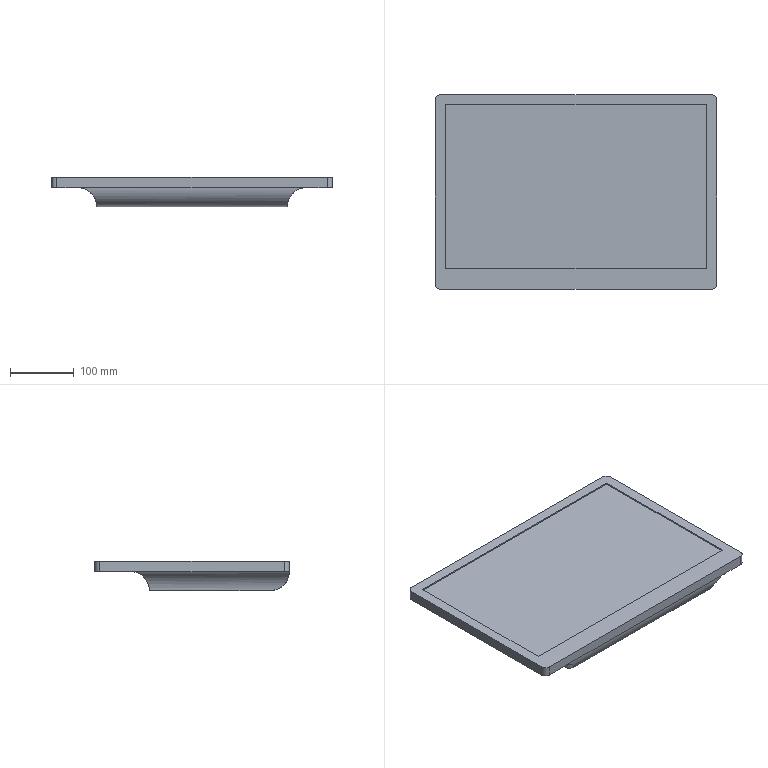Part | SolidWorks | features Fillet 3, ICE 2, Extrusion 1, HoleWzd 1 | 1 solid | 36 faces | box 442 x 306 x 46 mm | volume 4020857 mm3 | cylinder 16 | plane 12 | cone 8 | commonest cylinder face diameters 3.3 x8 16 x4 60 x4
STEP:
#1=CARTESIAN_POINT('',(51.65,41.,-19.9));
#2=VERTEX_POINT('',#1);
#3=CARTESIAN_POINT('',(48.35,41.,-19.9));
#4=VERTEX_POINT('',#3);
#5=CARTESIAN_POINT('',(50.,41.,-19.9));
#6=DIRECTION('',(0.,0.,-1.));
#7=DIRECTION('',(-1.,0.,0.));
#8=AXIS2_PLACEMENT_3D('',#5,#6,#7);
#9=CIRCLE('',#8,1.65);
#10=EDGE_CURVE('',#2,#4,#9,.T.);
#11=ORIENTED_EDGE('',*,*,#10,.F.);
#12=CARTESIAN_POINT('',(51.65,41.,-30.));
#13=VERTEX_POINT('',#12);
#14=CARTESIAN_POINT('',(51.65,41.,-30.));
#15=DIRECTION('',(0.,0.,-1.));
#16=VECTOR('',#15,1000.);
#17=LINE('',#14,#16);
#18=EDGE_CURVE('',#2,#13,#17,.T.);
#19=ORIENTED_EDGE('',*,*,#18,.T.);
#20=CARTESIAN_POINT('',(48.35,41.,-30.));
#21=VERTEX_POINT('',#20);
#22=CARTESIAN_POINT('',(50.,41.,-30.));
#23=DIRECTION('',(0.,0.,-1.));
#24=DIRECTION('',(-1.,0.,0.));
#25=AXIS2_PLACEMENT_3D('',#22,#23,#24);
#26=CIRCLE('',#25,1.65);
#27=EDGE_CURVE('',#13,#21,#26,.T.);
#28=ORIENTED_EDGE('',*,*,#27,.T.);
#29=CARTESIAN_POINT('',(48.35,41.,-30.));
#30=DIRECTION('',(0.,0.,-1.));
#31=VECTOR('',#30,1000.);
#32=LINE('',#29,#31);
#33=EDGE_CURVE('',#4,#21,#32,.T.);
#34=ORIENTED_EDGE('',*,*,#33,.F.);
#35=EDGE_LOOP('',(#11,#19,#28,#34));
#36=FACE_OUTER_BOUND('',#35,.T.);
#37=CARTESIAN_POINT('',(50.,41.,-30.));
#38=DIRECTION('',(0.,0.,-1.));
#39=DIRECTION('',(-1.,0.,0.));
#40=AXIS2_PLACEMENT_3D('',#37,#38,#39);
#41=CYLINDRICAL_SURFACE('',#40,1.65);
#42=ADVANCED_FACE('',(#36),#41,.F.);
#43=CARTESIAN_POINT('',(50.,41.,-18.909));
#44=VERTEX_POINT('',#43);
#45=CARTESIAN_POINT('',(48.35,41.,-19.9));
#46=DIRECTION('',(-0.8572,0.,-0.515));
#47=VECTOR('',#46,1000.);
#48=LINE('',#45,#47);
#49=EDGE_CURVE('',#44,#4,#48,.T.);
#50=ORIENTED_EDGE('',*,*,#49,.F.);
#51=CARTESIAN_POINT('',(51.65,41.,-19.9));
#52=DIRECTION('',(0.8572,0.,-0.515));
#53=VECTOR('',#52,1000.);
#54=LINE('',#51,#53);
#55=EDGE_CURVE('',#44,#2,#54,.T.);
#56=ORIENTED_EDGE('',*,*,#55,.T.);
#57=ORIENTED_EDGE('',*,*,#10,.T.);
#58=EDGE_LOOP('',(#50,#56,#57));
#59=FACE_OUTER_BOUND('',#58,.T.);
#60=CARTESIAN_POINT('',(50.,41.,-19.9));
#61=DIRECTION('',(0.,0.,-1.));
#62=DIRECTION('',(-1.,0.,0.));
#63=AXIS2_PLACEMENT_3D('',#60,#61,#62);
#64=CONICAL_SURFACE('',#63,1.65,1.03);
#65=ADVANCED_FACE('',(#59),#64,.F.);
#66=CARTESIAN_POINT('',(-48.35,41.,-19.9));
#67=VERTEX_POINT('',#66);
#68=CARTESIAN_POINT('',(-51.65,41.,-19.9));
#69=VERTEX_POINT('',#68);
#70=CARTESIAN_POINT('',(-50.,41.,-19.9));
#71=DIRECTION('',(0.,0.,-1.));
#72=DIRECTION('',(-1.,0.,0.));
#73=AXIS2_PLACEMENT_3D('',#70,#71,#72);
#74=CIRCLE('',#73,1.65);
#75=EDGE_CURVE('',#67,#69,#74,.T.);
#76=ORIENTED_EDGE('',*,*,#75,.F.);
#77=CARTESIAN_POINT('',(-48.35,41.,-30.));
#78=VERTEX_POINT('',#77);
#79=CARTESIAN_POINT('',(-48.35,41.,-30.));
#80=DIRECTION('',(0.,0.,-1.));
#81=VECTOR('',#80,1000.);
#82=LINE('',#79,#81);
#83=EDGE_CURVE('',#67,#78,#82,.T.);
#84=ORIENTED_EDGE('',*,*,#83,.T.);
#85=CARTESIAN_POINT('',(-51.65,41.,-30.));
#86=VERTEX_POINT('',#85);
#87=CARTESIAN_POINT('',(-50.,41.,-30.));
#88=DIRECTION('',(0.,0.,-1.));
#89=DIRECTION('',(-1.,0.,0.));
#90=AXIS2_PLACEMENT_3D('',#87,#88,#89);
#91=CIRCLE('',#90,1.65);
#92=EDGE_CURVE('',#78,#86,#91,.T.);
#93=ORIENTED_EDGE('',*,*,#92,.T.);
#94=CARTESIAN_POINT('',(-51.65,41.,-30.));
#95=DIRECTION('',(0.,0.,-1.));
#96=VECTOR('',#95,1000.);
#97=LINE('',#94,#96);
#98=EDGE_CURVE('',#69,#86,#97,.T.);
#99=ORIENTED_EDGE('',*,*,#98,.F.);
#100=EDGE_LOOP('',(#76,#84,#93,#99));
#101=FACE_OUTER_BOUND('',#100,.T.);
#102=CARTESIAN_POINT('',(-50.,41.,-30.));
#103=DIRECTION('',(0.,0.,-1.));
#104=DIRECTION('',(-1.,0.,0.));
#105=AXIS2_PLACEMENT_3D('',#102,#103,#104);
#106=CYLINDRICAL_SURFACE('',#105,1.65);
#107=ADVANCED_FACE('',(#101),#106,.F.);
#108=CARTESIAN_POINT('',(-50.,41.,-18.909));
#109=VERTEX_POINT('',#108);
#110=CARTESIAN_POINT('',(-51.65,41.,-19.9));
#111=DIRECTION('',(-0.8572,0.,-0.515));
#112=VECTOR('',#111,1000.);
#113=LINE('',#110,#112);
#114=EDGE_CURVE('',#109,#69,#113,.T.);
#115=ORIENTED_EDGE('',*,*,#114,.F.);
#116=CARTESIAN_POINT('',(-48.35,41.,-19.9));
#117=DIRECTION('',(0.8572,0.,-0.515));
#118=VECTOR('',#117,1000.);
#119=LINE('',#116,#118);
#120=EDGE_CURVE('',#109,#67,#119,.T.);
#121=ORIENTED_EDGE('',*,*,#120,.T.);
#122=ORIENTED_EDGE('',*,*,#75,.T.);
#123=EDGE_LOOP('',(#115,#121,#122));
#124=FACE_OUTER_BOUND('',#123,.T.);
#125=CARTESIAN_POINT('',(-50.,41.,-19.9));
#126=DIRECTION('',(0.,0.,-1.));
#127=DIRECTION('',(-1.,0.,0.));
#128=AXIS2_PLACEMENT_3D('',#125,#126,#127);
#129=CONICAL_SURFACE('',#128,1.65,1.03);
#130=ADVANCED_FACE('',(#124),#129,.F.);
#131=CARTESIAN_POINT('',(-48.35,-59.,-19.9));
#132=VERTEX_POINT('',#131);
#133=CARTESIAN_POINT('',(-51.65,-59.,-19.9));
#134=VERTEX_POINT('',#133);
#135=CARTESIAN_POINT('',(-50.,-59.,-19.9));
#136=DIRECTION('',(0.,0.,-1.));
#137=DIRECTION('',(-1.,0.,0.));
#138=AXIS2_PLACEMENT_3D('',#135,#136,#137);
#139=CIRCLE('',#138,1.65);
#140=EDGE_CURVE('',#132,#134,#139,.T.);
#141=ORIENTED_EDGE('',*,*,#140,.F.);
#142=CARTESIAN_POINT('',(-48.35,-59.,-30.));
#143=VERTEX_POINT('',#142);
#144=CARTESIAN_POINT('',(-48.35,-59.,-30.));
#145=DIRECTION('',(0.,0.,-1.));
#146=VECTOR('',#145,1000.);
#147=LINE('',#144,#146);
#148=EDGE_CURVE('',#132,#143,#147,.T.);
#149=ORIENTED_EDGE('',*,*,#148,.T.);
#150=CARTESIAN_POINT('',(-51.65,-59.,-30.));
#151=VERTEX_POINT('',#150);
#152=CARTESIAN_POINT('',(-50.,-59.,-30.));
#153=DIRECTION('',(0.,0.,-1.));
#154=DIRECTION('',(-1.,0.,0.));
#155=AXIS2_PLACEMENT_3D('',#152,#153,#154);
#156=CIRCLE('',#155,1.65);
#157=EDGE_CURVE('',#143,#151,#156,.T.);
#158=ORIENTED_EDGE('',*,*,#157,.T.);
#159=CARTESIAN_POINT('',(-51.65,-59.,-30.));
#160=DIRECTION('',(0.,0.,-1.));
#161=VECTOR('',#160,1000.);
#162=LINE('',#159,#161);
#163=EDGE_CURVE('',#134,#151,#162,.T.);
#164=ORIENTED_EDGE('',*,*,#163,.F.);
#165=EDGE_LOOP('',(#141,#149,#158,#164));
#166=FACE_OUTER_BOUND('',#165,.T.);
#167=CARTESIAN_POINT('',(-50.,-59.,-30.));
#168=DIRECTION('',(0.,0.,-1.));
#169=DIRECTION('',(-1.,0.,0.));
#170=AXIS2_PLACEMENT_3D('',#167,#168,#169);
#171=CYLINDRICAL_SURFACE('',#170,1.65);
#172=ADVANCED_FACE('',(#166),#171,.F.);
#173=CARTESIAN_POINT('',(-50.,-59.,-18.909));
#174=VERTEX_POINT('',#173);
#175=CARTESIAN_POINT('',(-51.65,-59.,-19.9));
#176=DIRECTION('',(-0.8572,0.,-0.515));
#177=VECTOR('',#176,1000.);
#178=LINE('',#175,#177);
#179=EDGE_CURVE('',#174,#134,#178,.T.);
#180=ORIENTED_EDGE('',*,*,#179,.F.);
#181=CARTESIAN_POINT('',(-48.35,-59.,-19.9));
#182=DIRECTION('',(0.8572,0.,-0.515));
#183=VECTOR('',#182,1000.);
#184=LINE('',#181,#183);
#185=EDGE_CURVE('',#174,#132,#184,.T.);
#186=ORIENTED_EDGE('',*,*,#185,.T.);
#187=ORIENTED_EDGE('',*,*,#140,.T.);
#188=EDGE_LOOP('',(#180,#186,#187));
#189=FACE_OUTER_BOUND('',#188,.T.);
#190=CARTESIAN_POINT('',(-50.,-59.,-19.9));
#191=DIRECTION('',(0.,0.,-1.));
#192=DIRECTION('',(-1.,0.,0.));
#193=AXIS2_PLACEMENT_3D('',#190,#191,#192);
#194=CONICAL_SURFACE('',#193,1.65,1.03);
#195=ADVANCED_FACE('',(#189),#194,.F.);
#196=CARTESIAN_POINT('',(51.65,-59.,-19.9));
#197=VERTEX_POINT('',#196);
#198=CARTESIAN_POINT('',(48.35,-59.,-19.9));
#199=VERTEX_POINT('',#198);
#200=CARTESIAN_POINT('',(50.,-59.,-19.9));
#201=DIRECTION('',(0.,0.,-1.));
#202=DIRECTION('',(-1.,0.,0.));
#203=AXIS2_PLACEMENT_3D('',#200,#201,#202);
#204=CIRCLE('',#203,1.65);
#205=EDGE_CURVE('',#197,#199,#204,.T.);
#206=ORIENTED_EDGE('',*,*,#205,.F.);
#207=CARTESIAN_POINT('',(51.65,-59.,-30.));
#208=VERTEX_POINT('',#207);
#209=CARTESIAN_POINT('',(51.65,-59.,-30.));
#210=DIRECTION('',(0.,0.,-1.));
#211=VECTOR('',#210,1000.);
#212=LINE('',#209,#211);
#213=EDGE_CURVE('',#197,#208,#212,.T.);
#214=ORIENTED_EDGE('',*,*,#213,.T.);
#215=CARTESIAN_POINT('',(48.35,-59.,-30.));
#216=VERTEX_POINT('',#215);
#217=CARTESIAN_POINT('',(50.,-59.,-30.));
#218=DIRECTION('',(0.,0.,-1.));
#219=DIRECTION('',(-1.,0.,0.));
#220=AXIS2_PLACEMENT_3D('',#217,#218,#219);
#221=CIRCLE('',#220,1.65);
#222=EDGE_CURVE('',#208,#216,#221,.T.);
#223=ORIENTED_EDGE('',*,*,#222,.T.);
#224=CARTESIAN_POINT('',(48.35,-59.,-30.));
#225=DIRECTION('',(0.,0.,-1.));
#226=VECTOR('',#225,1000.);
#227=LINE('',#224,#226);
#228=EDGE_CURVE('',#199,#216,#227,.T.);
#229=ORIENTED_EDGE('',*,*,#228,.F.);
#230=EDGE_LOOP('',(#206,#214,#223,#229));
#231=FACE_OUTER_BOUND('',#230,.T.);
#232=CARTESIAN_POINT('',(50.,-59.,-30.));
#233=DIRECTION('',(0.,0.,-1.));
#234=DIRECTION('',(-1.,0.,0.));
#235=AXIS2_PLACEMENT_3D('',#232,#233,#234);
#236=CYLINDRICAL_SURFACE('',#235,1.65);
#237=ADVANCED_FACE('',(#231),#236,.F.);
#238=CARTESIAN_POINT('',(50.,-59.,-18.909));
#239=VERTEX_POINT('',#238);
#240=CARTESIAN_POINT('',(48.35,-59.,-19.9));
#241=DIRECTION('',(-0.8572,0.,-0.515));
#242=VECTOR('',#241,1000.);
#243=LINE('',#240,#242);
#244=EDGE_CURVE('',#239,#199,#243,.T.);
#245=ORIENTED_EDGE('',*,*,#244,.F.);
#246=CARTESIAN_POINT('',(51.65,-59.,-19.9));
#247=DIRECTION('',(0.8572,0.,-0.515));
#248=VECTOR('',#247,1000.);
#249=LINE('',#246,#248);
#250=EDGE_CURVE('',#239,#197,#249,.T.);
#251=ORIENTED_EDGE('',*,*,#250,.T.);
#252=ORIENTED_EDGE('',*,*,#205,.T.);
#253=EDGE_LOOP('',(#245,#251,#252));
#254=FACE_OUTER_BOUND('',#253,.T.);
#255=CARTESIAN_POINT('',(50.,-59.,-19.9));
#256=DIRECTION('',(0.,0.,-1.));
#257=DIRECTION('',(-1.,0.,0.));
#258=AXIS2_PLACEMENT_3D('',#255,#256,#257);
#259=CONICAL_SURFACE('',#258,1.65,1.03);
#260=ADVANCED_FACE('',(#254),#259,.F.);
#261=CARTESIAN_POINT('',(-213.,-153.,0.));
#262=VERTEX_POINT('',#261);
#263=CARTESIAN_POINT('',(-180.,-153.,0.));
#264=VERTEX_POINT('',#263);
#265=CARTESIAN_POINT('',(-221.,-153.,0.));
#266=DIRECTION('',(1.,0.,0.));
#267=VECTOR('',#266,1000.);
#268=LINE('',#265,#267);
#269=EDGE_CURVE('',#262,#264,#268,.T.);
#270=ORIENTED_EDGE('',*,*,#269,.F.);
#271=CARTESIAN_POINT('',(-221.,-145.,0.));
#272=VERTEX_POINT('',#271);
#273=CARTESIAN_POINT('',(-213.,-145.,0.));
#274=DIRECTION('',(0.,0.,-1.));
#275=DIRECTION('',(1.,0.,0.));
#276=AXIS2_PLACEMENT_3D('',#273,#274,#275);
#277=CIRCLE('',#276,8.);
#278=EDGE_CURVE('',#262,#272,#277,.T.);
#279=ORIENTED_EDGE('',*,*,#278,.T.);
#280=CARTESIAN_POINT('',(-221.,145.,0.));
#281=VERTEX_POINT('',#280);
#282=CARTESIAN_POINT('',(-221.,153.,0.));
#283=DIRECTION('',(0.,-1.,0.));
#284=VECTOR('',#283,1000.);
#285=LINE('',#282,#284);
#286=EDGE_CURVE('',#281,#272,#285,.T.);
#287=ORIENTED_EDGE('',*,*,#286,.F.);
#288=CARTESIAN_POINT('',(-213.,153.,0.));
#289=VERTEX_POINT('',#288);
#290=CARTESIAN_POINT('',(-213.,145.,0.));
#291=DIRECTION('',(0.,0.,-1.));
#292=DIRECTION('',(1.,0.,0.));
#293=AXIS2_PLACEMENT_3D('',#290,#291,#292);
#294=CIRCLE('',#293,8.);
#295=EDGE_CURVE('',#281,#289,#294,.T.);
#296=ORIENTED_EDGE('',*,*,#295,.T.);
#297=CARTESIAN_POINT('',(213.,153.,0.));
#298=VERTEX_POINT('',#297);
#299=CARTESIAN_POINT('',(-221.,153.,0.));
#300=DIRECTION('',(-1.,0.,0.));
#301=VECTOR('',#300,1000.);
#302=LINE('',#299,#301);
#303=EDGE_CURVE('',#298,#289,#302,.T.);
#304=ORIENTED_EDGE('',*,*,#303,.F.);
#305=CARTESIAN_POINT('',(221.,145.,0.));
#306=VERTEX_POINT('',#305);
#307=CARTESIAN_POINT('',(213.,145.,0.));
#308=DIRECTION('',(0.,0.,-1.));
#309=DIRECTION('',(1.,0.,0.));
#310=AXIS2_PLACEMENT_3D('',#307,#308,#309);
#311=CIRCLE('',#310,8.);
#312=EDGE_CURVE('',#298,#306,#311,.T.);
#313=ORIENTED_EDGE('',*,*,#312,.T.);
#314=CARTESIAN_POINT('',(221.,-145.,0.));
#315=VERTEX_POINT('',#314);
#316=CARTESIAN_POINT('',(221.,153.,0.));
#317=DIRECTION('',(0.,1.,0.));
#318=VECTOR('',#317,1000.);
#319=LINE('',#316,#318);
#320=EDGE_CURVE('',#315,#306,#319,.T.);
#321=ORIENTED_EDGE('',*,*,#320,.F.);
#322=CARTESIAN_POINT('',(213.,-153.,0.));
#323=VERTEX_POINT('',#322);
#324=CARTESIAN_POINT('',(213.,-145.,0.));
#325=DIRECTION('',(0.,0.,-1.));
#326=DIRECTION('',(1.,0.,0.));
#327=AXIS2_PLACEMENT_3D('',#324,#325,#326);
#328=CIRCLE('',#327,8.);
#329=EDGE_CURVE('',#315,#323,#328,.T.);
#330=ORIENTED_EDGE('',*,*,#329,.T.);
#331=CARTESIAN_POINT('',(180.,-153.,0.));
#332=VERTEX_POINT('',#331);
#333=CARTESIAN_POINT('',(-221.,-153.,0.));
#334=DIRECTION('',(1.,0.,0.));
#335=VECTOR('',#334,1000.);
#336=LINE('',#333,#335);
#337=EDGE_CURVE('',#332,#323,#336,.T.);
#338=ORIENTED_EDGE('',*,*,#337,.F.);
#339=CARTESIAN_POINT('',(180.,97.,0.));
#340=VERTEX_POINT('',#339);
#341=CARTESIAN_POINT('',(180.,67.,0.));
#342=DIRECTION('',(0.,1.,0.));
#343=VECTOR('',#342,1000.);
#344=LINE('',#341,#343);
#345=EDGE_CURVE('',#332,#340,#344,.T.);
#346=ORIENTED_EDGE('',*,*,#345,.T.);
#347=CARTESIAN_POINT('',(-180.,97.,0.));
#348=VERTEX_POINT('',#347);
#349=CARTESIAN_POINT('',(-150.,97.,0.));
#350=DIRECTION('',(-1.,0.,0.));
#351=VECTOR('',#350,1000.);
#352=LINE('',#349,#351);
#353=EDGE_CURVE('',#340,#348,#352,.T.);
#354=ORIENTED_EDGE('',*,*,#353,.T.);
#355=CARTESIAN_POINT('',(-180.,-153.,0.));
#356=DIRECTION('',(0.,-1.,0.));
#357=VECTOR('',#356,1000.);
#358=LINE('',#355,#357);
#359=EDGE_CURVE('',#348,#264,#358,.T.);
#360=ORIENTED_EDGE('',*,*,#359,.T.);
#361=EDGE_LOOP('',(#270,#279,#287,#296,#304,#313,#321,#330,#338,#346,#354,#360));
#362=FACE_OUTER_BOUND('',#361,.T.);
#363=CARTESIAN_POINT('',(0.,0.,0.));
#364=DIRECTION('',(0.,0.,1.));
#365=DIRECTION('',(1.,0.,0.));
#366=AXIS2_PLACEMENT_3D('',#363,#364,#365);
#367=PLANE('',#366);
#368=ADVANCED_FACE('',(#362),#367,.F.);
#369=CARTESIAN_POINT('',(221.,-145.,16.));
#370=VERTEX_POINT('',#369);
#371=CARTESIAN_POINT('',(221.,145.,16.));
#372=VERTEX_POINT('',#371);
#373=CARTESIAN_POINT('',(221.,153.,16.));
#374=DIRECTION('',(0.,1.,0.));
#375=VECTOR('',#374,1000.);
#376=LINE('',#373,#375);
#377=EDGE_CURVE('',#370,#372,#376,.T.);
#378=ORIENTED_EDGE('',*,*,#377,.F.);
#379=CARTESIAN_POINT('',(221.,-145.,16.));
#380=DIRECTION('',(0.,0.,-1.));
#381=VECTOR('',#380,1000.);
#382=LINE('',#379,#381);
#383=EDGE_CURVE('',#370,#315,#382,.T.);
#384=ORIENTED_EDGE('',*,*,#383,.T.);
#385=ORIENTED_EDGE('',*,*,#320,.T.);
#386=CARTESIAN_POINT('',(221.,145.,16.));
#387=DIRECTION('',(0.,0.,1.));
#388=VECTOR('',#387,1000.);
#389=LINE('',#386,#388);
#390=EDGE_CURVE('',#306,#372,#389,.T.);
#391=ORIENTED_EDGE('',*,*,#390,.T.);
#392=EDGE_LOOP('',(#378,#384,#385,#391));
#393=FACE_OUTER_BOUND('',#392,.T.);
#394=CARTESIAN_POINT('',(221.,153.,16.));
#395=DIRECTION('',(-1.,0.,0.));
#396=DIRECTION('',(0.,-1.,0.));
#397=AXIS2_PLACEMENT_3D('',#394,#395,#396);
#398=PLANE('',#397);
#399=ADVANCED_FACE('',(#393),#398,.F.);
#400=CARTESIAN_POINT('',(213.,153.,16.));
#401=VERTEX_POINT('',#400);
#402=CARTESIAN_POINT('',(-213.,153.,16.));
#403=VERTEX_POINT('',#402);
#404=CARTESIAN_POINT('',(-221.,153.,16.));
#405=DIRECTION('',(-1.,0.,0.));
#406=VECTOR('',#405,1000.);
#407=LINE('',#404,#406);
#408=EDGE_CURVE('',#401,#403,#407,.T.);
#409=ORIENTED_EDGE('',*,*,#408,.F.);
#410=CARTESIAN_POINT('',(213.,153.,16.));
#411=DIRECTION('',(0.,0.,-1.));
#412=VECTOR('',#411,1000.);
#413=LINE('',#410,#412);
#414=EDGE_CURVE('',#401,#298,#413,.T.);
#415=ORIENTED_EDGE('',*,*,#414,.T.);
#416=ORIENTED_EDGE('',*,*,#303,.T.);
#417=CARTESIAN_POINT('',(-213.,153.,16.));
#418=DIRECTION('',(0.,0.,1.));
#419=VECTOR('',#418,1000.);
#420=LINE('',#417,#419);
#421=EDGE_CURVE('',#289,#403,#420,.T.);
#422=ORIENTED_EDGE('',*,*,#421,.T.);
#423=EDGE_LOOP('',(#409,#415,#416,#422));
#424=FACE_OUTER_BOUND('',#423,.T.);
#425=CARTESIAN_POINT('',(-221.,153.,16.));
#426=DIRECTION('',(0.,-1.,0.));
#427=DIRECTION('',(0.,0.,-1.));
#428=AXIS2_PLACEMENT_3D('',#425,#426,#427);
#429=PLANE('',#428);
#430=ADVANCED_FACE('',(#424),#429,.F.);
#431=ORIENTED_EDGE('',*,*,#286,.T.);
#432=CARTESIAN_POINT('',(-221.,-145.,16.));
#433=VERTEX_POINT('',#432);
#434=CARTESIAN_POINT('',(-221.,-145.,16.));
#435=DIRECTION('',(0.,0.,1.));
#436=VECTOR('',#435,1000.);
#437=LINE('',#434,#436);
#438=EDGE_CURVE('',#272,#433,#437,.T.);
#439=ORIENTED_EDGE('',*,*,#438,.T.);
#440=CARTESIAN_POINT('',(-221.,145.,16.));
#441=VERTEX_POINT('',#440);
#442=CARTESIAN_POINT('',(-221.,153.,16.));
#443=DIRECTION('',(0.,-1.,0.));
#444=VECTOR('',#443,1000.);
#445=LINE('',#442,#444);
#446=EDGE_CURVE('',#441,#433,#445,.T.);
#447=ORIENTED_EDGE('',*,*,#446,.F.);
#448=CARTESIAN_POINT('',(-221.,145.,16.));
#449=DIRECTION('',(0.,0.,-1.));
#450=VECTOR('',#449,1000.);
#451=LINE('',#448,#450);
#452=EDGE_CURVE('',#441,#281,#451,.T.);
#453=ORIENTED_EDGE('',*,*,#452,.T.);
#454=EDGE_LOOP('',(#431,#439,#447,#453));
#455=FACE_OUTER_BOUND('',#454,.T.);
#456=CARTESIAN_POINT('',(-221.,153.,16.));
#457=DIRECTION('',(1.,0.,0.));
#458=DIRECTION('',(0.,1.,0.));
#459=AXIS2_PLACEMENT_3D('',#456,#457,#458);
#460=PLANE('',#459);
#461=ADVANCED_FACE('',(#455),#460,.F.);
#462=CARTESIAN_POINT('',(-213.,-153.,16.));
#463=VERTEX_POINT('',#462);
#464=CARTESIAN_POINT('',(213.,-153.,16.));
#465=VERTEX_POINT('',#464);
#466=CARTESIAN_POINT('',(-221.,-153.,16.));
#467=DIRECTION('',(1.,0.,0.));
#468=VECTOR('',#467,1000.);
#469=LINE('',#466,#468);
#470=EDGE_CURVE('',#463,#465,#469,.T.);
#471=ORIENTED_EDGE('',*,*,#470,.F.);
#472=CARTESIAN_POINT('',(-213.,-153.,16.));
#473=DIRECTION('',(0.,0.,-1.));
#474=VECTOR('',#473,1000.);
#475=LINE('',#472,#474);
#476=EDGE_CURVE('',#463,#262,#475,.T.);
#477=ORIENTED_EDGE('',*,*,#476,.T.);
#478=ORIENTED_EDGE('',*,*,#269,.T.);
#479=CARTESIAN_POINT('',(-221.,-153.,0.));
#480=DIRECTION('',(1.,0.,0.));
#481=VECTOR('',#480,1000.);
#482=LINE('',#479,#481);
#483=EDGE_CURVE('',#264,#332,#482,.T.);
#484=ORIENTED_EDGE('',*,*,#483,.T.);
#485=ORIENTED_EDGE('',*,*,#337,.T.);
#486=CARTESIAN_POINT('',(213.,-153.,16.));
#487=DIRECTION('',(0.,0.,1.));
#488=VECTOR('',#487,1000.);
#489=LINE('',#486,#488);
#490=EDGE_CURVE('',#323,#465,#489,.T.);
#491=ORIENTED_EDGE('',*,*,#490,.T.);
#492=EDGE_LOOP('',(#471,#477,#478,#484,#485,#491));
#493=FACE_OUTER_BOUND('',#492,.T.);
#494=CARTESIAN_POINT('',(-221.,-153.,16.));
#495=DIRECTION('',(0.,1.,0.));
#496=DIRECTION('',(0.,0.,1.));
#497=AXIS2_PLACEMENT_3D('',#494,#495,#496);
#498=PLANE('',#497);
#499=ADVANCED_FACE('',(#493),#498,.F.);
#500=CARTESIAN_POINT('',(205.,-121.,16.));
#501=VERTEX_POINT('',#500);
#502=CARTESIAN_POINT('',(205.,137.,16.));
#503=VERTEX_POINT('',#502);
#504=CARTESIAN_POINT('',(205.,137.,16.));
#505=DIRECTION('',(0.,1.,0.));
#506=VECTOR('',#505,1000.);
#507=LINE('',#504,#506);
#508=EDGE_CURVE('',#501,#503,#507,.T.);
#509=ORIENTED_EDGE('',*,*,#508,.F.);
#510=CARTESIAN_POINT('',(-205.,-121.,16.));
#511=VERTEX_POINT('',#510);
#512=CARTESIAN_POINT('',(-205.,-121.,16.));
#513=DIRECTION('',(1.,0.,0.));
#514=VECTOR('',#513,1000.);
#515=LINE('',#512,#514);
#516=EDGE_CURVE('',#511,#501,#515,.T.);
#517=ORIENTED_EDGE('',*,*,#516,.F.);
#518=CARTESIAN_POINT('',(-205.,137.,16.));
#519=VERTEX_POINT('',#518);
#520=CARTESIAN_POINT('',(-205.,137.,16.));
#521=DIRECTION('',(0.,-1.,0.));
#522=VECTOR('',#521,1000.);
#523=LINE('',#520,#522);
#524=EDGE_CURVE('',#519,#511,#523,.T.);
#525=ORIENTED_EDGE('',*,*,#524,.F.);
#526=CARTESIAN_POINT('',(-205.,137.,16.));
#527=DIRECTION('',(-1.,0.,0.));
#528=VECTOR('',#527,1000.);
#529=LINE('',#526,#528);
#530=EDGE_CURVE('',#503,#519,#529,.T.);
#531=ORIENTED_EDGE('',*,*,#530,.F.);
#532=EDGE_LOOP('',(#509,#517,#525,#531));
#533=FACE_BOUND('',#532,.T.);
#534=ORIENTED_EDGE('',*,*,#446,.T.);
#535=CARTESIAN_POINT('',(-213.,-145.,16.));
#536=DIRECTION('',(0.,0.,1.));
#537=DIRECTION('',(1.,0.,0.));
#538=AXIS2_PLACEMENT_3D('',#535,#536,#537);
#539=CIRCLE('',#538,8.);
#540=EDGE_CURVE('',#433,#463,#539,.T.);
#541=ORIENTED_EDGE('',*,*,#540,.T.);
#542=ORIENTED_EDGE('',*,*,#470,.T.);
#543=CARTESIAN_POINT('',(213.,-145.,16.));
#544=DIRECTION('',(0.,0.,1.));
#545=DIRECTION('',(1.,0.,0.));
#546=AXIS2_PLACEMENT_3D('',#543,#544,#545);
#547=CIRCLE('',#546,8.);
#548=EDGE_CURVE('',#465,#370,#547,.T.);
#549=ORIENTED_EDGE('',*,*,#548,.T.);
#550=ORIENTED_EDGE('',*,*,#377,.T.);
#551=CARTESIAN_POINT('',(213.,145.,16.));
#552=DIRECTION('',(0.,0.,1.));
#553=DIRECTION('',(1.,0.,0.));
#554=AXIS2_PLACEMENT_3D('',#551,#552,#553);
#555=CIRCLE('',#554,8.);
#556=EDGE_CURVE('',#372,#401,#555,.T.);
#557=ORIENTED_EDGE('',*,*,#556,.T.);
#558=ORIENTED_EDGE('',*,*,#408,.T.);
#559=CARTESIAN_POINT('',(-213.,145.,16.));
#560=DIRECTION('',(0.,0.,1.));
#561=DIRECTION('',(1.,0.,0.));
#562=AXIS2_PLACEMENT_3D('',#559,#560,#561);
#563=CIRCLE('',#562,8.);
#564=EDGE_CURVE('',#403,#441,#563,.T.);
#565=ORIENTED_EDGE('',*,*,#564,.T.);
#566=EDGE_LOOP('',(#534,#541,#542,#549,#550,#557,#558,#565));
#567=FACE_OUTER_BOUND('',#566,.T.);
#568=CARTESIAN_POINT('',(0.,0.,16.));
#569=DIRECTION('',(0.,0.,1.));
#570=DIRECTION('',(1.,0.,0.));
#571=AXIS2_PLACEMENT_3D('',#568,#569,#570);
#572=PLANE('',#571);
#573=ADVANCED_FACE('',(#533,#567),#572,.T.);
#574=CARTESIAN_POINT('',(50.,41.,-30.));
#575=DIRECTION('',(0.,0.,-1.));
#576=DIRECTION('',(-1.,0.,0.));
#577=AXIS2_PLACEMENT_3D('',#574,#575,#576);
#578=CIRCLE('',#577,1.65);
#579=EDGE_CURVE('',#21,#13,#578,.T.);
#580=ORIENTED_EDGE('',*,*,#579,.F.);
#581=ORIENTED_EDGE('',*,*,#27,.F.);
#582=EDGE_LOOP('',(#580,#581));
#583=FACE_BOUND('',#582,.T.);
#584=CARTESIAN_POINT('',(-50.,41.,-30.));
#585=DIRECTION('',(0.,0.,-1.));
#586=DIRECTION('',(-1.,0.,0.));
#587=AXIS2_PLACEMENT_3D('',#584,#585,#586);
#588=CIRCLE('',#587,1.65);
#589=EDGE_CURVE('',#86,#78,#588,.T.);
#590=ORIENTED_EDGE('',*,*,#589,.F.);
#591=ORIENTED_EDGE('',*,*,#92,.F.);
#592=EDGE_LOOP('',(#590,#591));
#593=FACE_BOUND('',#592,.T.);
#594=CARTESIAN_POINT('',(-50.,-59.,-30.));
#595=DIRECTION('',(0.,0.,-1.));
#596=DIRECTION('',(-1.,0.,0.));
#597=AXIS2_PLACEMENT_3D('',#594,#595,#596);
#598=CIRCLE('',#597,1.65);
#599=EDGE_CURVE('',#151,#143,#598,.T.);
#600=ORIENTED_EDGE('',*,*,#599,.F.);
#601=ORIENTED_EDGE('',*,*,#157,.F.);
#602=EDGE_LOOP('',(#600,#601));
#603=FACE_BOUND('',#602,.T.);
#604=CARTESIAN_POINT('',(50.,-59.,-30.));
#605=DIRECTION('',(0.,0.,-1.));
#606=DIRECTION('',(-1.,0.,0.));
#607=AXIS2_PLACEMENT_3D('',#604,#605,#606);
#608=CIRCLE('',#607,1.65);
#609=EDGE_CURVE('',#216,#208,#608,.T.);
#610=ORIENTED_EDGE('',*,*,#609,.F.);
#611=ORIENTED_EDGE('',*,*,#222,.F.);
#612=EDGE_LOOP('',(#610,#611));
#613=FACE_BOUND('',#612,.T.);
#614=CARTESIAN_POINT('',(150.,67.,-30.));
#615=VERTEX_POINT('',#614);
#616=CARTESIAN_POINT('',(150.,-123.,-30.));
#617=VERTEX_POINT('',#616);
#618=CARTESIAN_POINT('',(150.,-153.,-30.));
#619=DIRECTION('',(0.,-1.,0.));
#620=VECTOR('',#619,1000.);
#621=LINE('',#618,#620);
#622=EDGE_CURVE('',#615,#617,#621,.T.);
#623=ORIENTED_EDGE('',*,*,#622,.T.);
#624=CARTESIAN_POINT('',(-150.,-123.,-30.));
#625=VERTEX_POINT('',#624);
#626=CARTESIAN_POINT('',(0.,-123.,-30.));
#627=DIRECTION('',(-1.,0.,0.));
#628=VECTOR('',#627,1000.);
#629=LINE('',#626,#628);
#630=EDGE_CURVE('',#617,#625,#629,.T.);
#631=ORIENTED_EDGE('',*,*,#630,.T.);
#632=CARTESIAN_POINT('',(-150.,67.,-30.));
#633=VERTEX_POINT('',#632);
#634=CARTESIAN_POINT('',(-150.,-153.,-30.));
#635=DIRECTION('',(0.,1.,0.));
#636=VECTOR('',#635,1000.);
#637=LINE('',#634,#636);
#638=EDGE_CURVE('',#625,#633,#637,.T.);
#639=ORIENTED_EDGE('',*,*,#638,.T.);
#640=CARTESIAN_POINT('',(150.,67.,-30.));
#641=DIRECTION('',(1.,0.,0.));
#642=VECTOR('',#641,1000.);
#643=LINE('',#640,#642);
#644=EDGE_CURVE('',#633,#615,#643,.T.);
#645=ORIENTED_EDGE('',*,*,#644,.T.);
#646=EDGE_LOOP('',(#623,#631,#639,#645));
#647=FACE_OUTER_BOUND('',#646,.T.);
#648=CARTESIAN_POINT('',(0.,0.,-30.));
#649=DIRECTION('',(0.,0.,1.));
#650=DIRECTION('',(1.,0.,0.));
#651=AXIS2_PLACEMENT_3D('',#648,#649,#650);
#652=PLANE('',#651);
#653=ADVANCED_FACE('',(#583,#593,#603,#613,#647),#652,.F.);
#654=ORIENTED_EDGE('',*,*,#638,.F.);
#655=CARTESIAN_POINT('',(-150.,-123.,-30.));
#656=CARTESIAN_POINT('',(-150.,-124.343,-30.));
#657=CARTESIAN_POINT('',(-150.,-125.671,-29.91));
#658=CARTESIAN_POINT('',(-150.003,-128.298,-29.558));
#659=CARTESIAN_POINT('',(-150.006,-129.597,-29.296));
#660=CARTESIAN_POINT('',(-150.025,-131.523,-28.771));
#661=CARTESIAN_POINT('',(-150.033,-132.162,-28.575));
#662=CARTESIAN_POINT('',(-150.057,-133.431,-28.136));
#663=CARTESIAN_POINT('',(-150.073,-134.055,-27.897));
#664=CARTESIAN_POINT('',(-150.134,-135.893,-27.121));
#665=CARTESIAN_POINT('',(-150.194,-137.075,-26.526));
#666=CARTESIAN_POINT('',(-150.381,-139.351,-25.187));
#667=CARTESIAN_POINT('',(-150.507,-140.445,-24.442));
#668=CARTESIAN_POINT('',(-150.865,-142.543,-22.8));
#669=CARTESIAN_POINT('',(-151.092,-143.519,-21.923));
#670=CARTESIAN_POINT('',(-151.671,-145.325,-20.082));
#671=CARTESIAN_POINT('',(-152.023,-146.155,-19.116));
#672=CARTESIAN_POINT('',(-152.672,-147.295,-17.612));
#673=CARTESIAN_POINT('',(-152.909,-147.658,-17.099));
#674=CARTESIAN_POINT('',(-153.427,-148.344,-16.064));
#675=CARTESIAN_POINT('',(-153.704,-148.664,-15.547));
#676=CARTESIAN_POINT('',(-154.594,-149.559,-14.002));
#677=CARTESIAN_POINT('',(-155.265,-150.07,-12.978));
#678=CARTESIAN_POINT('',(-156.397,-150.726,-11.471));
#679=CARTESIAN_POINT('',(-156.796,-150.926,-10.974));
#680=CARTESIAN_POINT('',(-157.638,-151.292,-9.99));
#681=CARTESIAN_POINT('',(-158.077,-151.457,-9.51));
#682=CARTESIAN_POINT('',(-159.441,-151.899,-8.113));
#683=CARTESIAN_POINT('',(-160.416,-152.126,-7.236));
#684=CARTESIAN_POINT('',(-161.975,-152.395,-6.01));
#685=CARTESIAN_POINT('',(-162.511,-152.472,-5.616));
#686=CARTESIAN_POINT('',(-163.616,-152.606,-4.86));
#687=CARTESIAN_POINT('',(-164.178,-152.662,-4.503));
#688=CARTESIAN_POINT('',(-165.897,-152.804,-3.488));
#689=CARTESIAN_POINT('',(-167.084,-152.865,-2.89));
#690=CARTESIAN_POINT('',(-168.924,-152.927,-2.112));
#691=CARTESIAN_POINT('',(-169.547,-152.942,-1.872));
#692=CARTESIAN_POINT('',(-170.814,-152.967,-1.433));
#693=CARTESIAN_POINT('',(-171.457,-152.975,-1.234));
#694=CARTESIAN_POINT('',(-173.39,-152.994,-0.7069));
#695=CARTESIAN_POINT('',(-174.692,-152.997,-0.4434));
#696=CARTESIAN_POINT('',(-177.325,-153.,-0.08996));
#697=CARTESIAN_POINT('',(-178.656,-153.,0.));
#698=CARTESIAN_POINT('',(-180.,-153.,0.));
#699=B_SPLINE_CURVE_WITH_KNOTS('',3,(#655,#656,#657,#658,#659,#660,#661,#662,#663,#664,#665,#666,#667,#668,#669,#670,#671,#672,#673,#674,#675,#676,#677,#678,#679,#680,#681,#682,#683,#684,#685,#686,#687,#688,#689,#690,#691,#692,#693,#694,#695,#696,#697,#698),.UNSPECIFIED.,.F.,.F.,(4,2,2,2,2,2,2,2,2,2,2,2,2,2,2,2,2,2,2,2,2,4),(0.,0.003973,0.007947,0.009933,0.01192,0.01589,0.01987,0.02384,0.02781,0.0298,0.03179,0.03576,0.03775,0.03973,0.04371,0.04569,0.04768,0.05165,0.05364,0.05563,0.0596,0.06357),.UNSPECIFIED.);
#700=EDGE_CURVE('',#625,#264,#699,.T.);
#701=ORIENTED_EDGE('',*,*,#700,.T.);
#702=ORIENTED_EDGE('',*,*,#359,.F.);
#703=CARTESIAN_POINT('',(-150.,67.,-30.));
#704=CARTESIAN_POINT('',(-150.,67.,-12.426));
#705=CARTESIAN_POINT('',(-162.426,79.426,0.));
#706=CARTESIAN_POINT('',(-180.,97.,0.));
#707=(BOUNDED_CURVE()B_SPLINE_CURVE(3,(#703,#704,#705,#706),.UNSPECIFIED.,.F.,.F.)B_SPLINE_CURVE_WITH_KNOTS((4,4),(3.142,4.712),.UNSPECIFIED.)CURVE()GEOMETRIC_REPRESENTATION_ITEM()RATIONAL_B_SPLINE_CURVE((1.,0.8047,0.8047,1.))REPRESENTATION_ITEM(''));
#708=EDGE_CURVE('',#633,#348,#707,.T.);
#709=ORIENTED_EDGE('',*,*,#708,.F.);
#710=EDGE_LOOP('',(#654,#701,#702,#709));
#711=FACE_OUTER_BOUND('',#710,.T.);
#712=CARTESIAN_POINT('',(-180.,-153.,-30.));
#713=DIRECTION('',(0.,-1.,0.));
#714=DIRECTION('',(0.,0.,-1.));
#715=AXIS2_PLACEMENT_3D('',#712,#713,#714);
#716=CYLINDRICAL_SURFACE('',#715,30.);
#717=ADVANCED_FACE('',(#711),#716,.F.);
#718=ORIENTED_EDGE('',*,*,#708,.T.);
#719=ORIENTED_EDGE('',*,*,#353,.F.);
#720=CARTESIAN_POINT('',(150.,67.,-30.));
#721=CARTESIAN_POINT('',(150.,67.,-12.426));
#722=CARTESIAN_POINT('',(162.426,79.426,0.));
#723=CARTESIAN_POINT('',(180.,97.,0.));
#724=(BOUNDED_CURVE()B_SPLINE_CURVE(3,(#720,#721,#722,#723),.UNSPECIFIED.,.F.,.F.)B_SPLINE_CURVE_WITH_KNOTS((4,4),(0.,1.571),.UNSPECIFIED.)CURVE()GEOMETRIC_REPRESENTATION_ITEM()RATIONAL_B_SPLINE_CURVE((1.,0.8047,0.8047,1.))REPRESENTATION_ITEM(''));
#725=EDGE_CURVE('',#615,#340,#724,.T.);
#726=ORIENTED_EDGE('',*,*,#725,.F.);
#727=ORIENTED_EDGE('',*,*,#644,.F.);
#728=EDGE_LOOP('',(#718,#719,#726,#727));
#729=FACE_OUTER_BOUND('',#728,.T.);
#730=CARTESIAN_POINT('',(150.,97.,-30.));
#731=DIRECTION('',(-1.,0.,0.));
#732=DIRECTION('',(0.,0.,1.));
#733=AXIS2_PLACEMENT_3D('',#730,#731,#732);
#734=CYLINDRICAL_SURFACE('',#733,30.);
#735=ADVANCED_FACE('',(#729),#734,.F.);
#736=ORIENTED_EDGE('',*,*,#345,.F.);
#737=CARTESIAN_POINT('',(180.,-153.,0.));
#738=CARTESIAN_POINT('',(178.657,-153.,0.));
#739=CARTESIAN_POINT('',(177.329,-153.,-0.08979));
#740=CARTESIAN_POINT('',(174.702,-152.997,-0.4418));
#741=CARTESIAN_POINT('',(173.403,-152.994,-0.7041));
#742=CARTESIAN_POINT('',(171.477,-152.975,-1.229));
#743=CARTESIAN_POINT('',(170.838,-152.967,-1.425));
#744=CARTESIAN_POINT('',(169.569,-152.943,-1.864));
#745=CARTESIAN_POINT('',(168.945,-152.927,-2.103));
#746=CARTESIAN_POINT('',(167.107,-152.866,-2.879));
#747=CARTESIAN_POINT('',(165.925,-152.806,-3.474));
#748=CARTESIAN_POINT('',(163.649,-152.619,-4.813));
#749=CARTESIAN_POINT('',(162.555,-152.493,-5.558));
#750=CARTESIAN_POINT('',(160.457,-152.135,-7.2));
#751=CARTESIAN_POINT('',(159.481,-151.908,-8.077));
#752=CARTESIAN_POINT('',(157.675,-151.329,-9.918));
#753=CARTESIAN_POINT('',(156.845,-150.977,-10.884));
#754=CARTESIAN_POINT('',(155.705,-150.328,-12.388));
#755=CARTESIAN_POINT('',(155.342,-150.091,-12.901));
#756=CARTESIAN_POINT('',(154.656,-149.573,-13.936));
#757=CARTESIAN_POINT('',(154.336,-149.296,-14.453));
#758=CARTESIAN_POINT('',(153.441,-148.406,-15.998));
#759=CARTESIAN_POINT('',(152.93,-147.735,-17.022));
#760=CARTESIAN_POINT('',(152.274,-146.603,-18.529));
#761=CARTESIAN_POINT('',(152.074,-146.204,-19.026));
#762=CARTESIAN_POINT('',(151.708,-145.362,-20.01));
#763=CARTESIAN_POINT('',(151.543,-144.923,-20.49));
#764=CARTESIAN_POINT('',(151.101,-143.559,-21.887));
#765=CARTESIAN_POINT('',(150.874,-142.584,-22.764));
#766=CARTESIAN_POINT('',(150.605,-141.025,-23.99));
#767=CARTESIAN_POINT('',(150.528,-140.489,-24.384));
#768=CARTESIAN_POINT('',(150.394,-139.384,-25.14));
#769=CARTESIAN_POINT('',(150.338,-138.822,-25.497));
#770=CARTESIAN_POINT('',(150.196,-137.103,-26.512));
#771=CARTESIAN_POINT('',(150.135,-135.916,-27.11));
#772=CARTESIAN_POINT('',(150.073,-134.076,-27.888));
#773=CARTESIAN_POINT('',(150.058,-133.453,-28.128));
#774=CARTESIAN_POINT('',(150.033,-132.186,-28.567));
#775=CARTESIAN_POINT('',(150.025,-131.543,-28.766));
#776=CARTESIAN_POINT('',(150.006,-129.61,-29.293));
#777=CARTESIAN_POINT('',(150.003,-128.308,-29.557));
#778=CARTESIAN_POINT('',(150.,-125.675,-29.91));
#779=CARTESIAN_POINT('',(150.,-124.344,-30.));
#780=CARTESIAN_POINT('',(150.,-123.,-30.));
#781=B_SPLINE_CURVE_WITH_KNOTS('',3,(#737,#738,#739,#740,#741,#742,#743,#744,#745,#746,#747,#748,#749,#750,#751,#752,#753,#754,#755,#756,#757,#758,#759,#760,#761,#762,#763,#764,#765,#766,#767,#768,#769,#770,#771,#772,#773,#774,#775,#776,#777,#778,#779,#780),.UNSPECIFIED.,.F.,.F.,(4,2,2,2,2,2,2,2,2,2,2,2,2,2,2,2,2,2,2,2,2,4),(0.,0.003973,0.007947,0.009933,0.01192,0.01589,0.01987,0.02384,0.02781,0.0298,0.03179,0.03576,0.03775,0.03973,0.04371,0.04569,0.04768,0.05165,0.05364,0.05563,0.0596,0.06357),.UNSPECIFIED.);
#782=EDGE_CURVE('',#332,#617,#781,.T.);
#783=ORIENTED_EDGE('',*,*,#782,.T.);
#784=ORIENTED_EDGE('',*,*,#622,.F.);
#785=ORIENTED_EDGE('',*,*,#725,.T.);
#786=EDGE_LOOP('',(#736,#783,#784,#785));
#787=FACE_OUTER_BOUND('',#786,.T.);
#788=CARTESIAN_POINT('',(180.,-153.,-30.));
#789=DIRECTION('',(0.,1.,0.));
#790=DIRECTION('',(0.,0.,1.));
#791=AXIS2_PLACEMENT_3D('',#788,#789,#790);
#792=CYLINDRICAL_SURFACE('',#791,30.);
#793=ADVANCED_FACE('',(#787),#792,.F.);
#794=ORIENTED_EDGE('',*,*,#782,.F.);
#795=ORIENTED_EDGE('',*,*,#483,.F.);
#796=ORIENTED_EDGE('',*,*,#700,.F.);
#797=ORIENTED_EDGE('',*,*,#630,.F.);
#798=EDGE_LOOP('',(#794,#795,#796,#797));
#799=FACE_OUTER_BOUND('',#798,.T.);
#800=CARTESIAN_POINT('',(0.,-123.,0.));
#801=DIRECTION('',(-1.,0.,0.));
#802=DIRECTION('',(0.,0.,1.));
#803=AXIS2_PLACEMENT_3D('',#800,#801,#802);
#804=CYLINDRICAL_SURFACE('',#803,30.);
#805=ADVANCED_FACE('',(#799),#804,.T.);
#806=ORIENTED_EDGE('',*,*,#250,.F.);
#807=ORIENTED_EDGE('',*,*,#244,.T.);
#808=CARTESIAN_POINT('',(50.,-59.,-19.9));
#809=DIRECTION('',(0.,0.,-1.));
#810=DIRECTION('',(-1.,0.,0.));
#811=AXIS2_PLACEMENT_3D('',#808,#809,#810);
#812=CIRCLE('',#811,1.65);
#813=EDGE_CURVE('',#199,#197,#812,.T.);
#814=ORIENTED_EDGE('',*,*,#813,.T.);
#815=EDGE_LOOP('',(#806,#807,#814));
#816=FACE_OUTER_BOUND('',#815,.T.);
#817=CARTESIAN_POINT('',(50.,-59.,-19.9));
#818=DIRECTION('',(0.,0.,-1.));
#819=DIRECTION('',(-1.,0.,0.));
#820=AXIS2_PLACEMENT_3D('',#817,#818,#819);
#821=CONICAL_SURFACE('',#820,1.65,1.03);
#822=ADVANCED_FACE('',(#816),#821,.F.);
#823=ORIENTED_EDGE('',*,*,#213,.F.);
#824=ORIENTED_EDGE('',*,*,#813,.F.);
#825=ORIENTED_EDGE('',*,*,#228,.T.);
#826=ORIENTED_EDGE('',*,*,#609,.T.);
#827=EDGE_LOOP('',(#823,#824,#825,#826));
#828=FACE_OUTER_BOUND('',#827,.T.);
#829=CARTESIAN_POINT('',(50.,-59.,-30.));
#830=DIRECTION('',(0.,0.,-1.));
#831=DIRECTION('',(-1.,0.,0.));
#832=AXIS2_PLACEMENT_3D('',#829,#830,#831);
#833=CYLINDRICAL_SURFACE('',#832,1.65);
#834=ADVANCED_FACE('',(#828),#833,.F.);
#835=ORIENTED_EDGE('',*,*,#185,.F.);
#836=ORIENTED_EDGE('',*,*,#179,.T.);
#837=CARTESIAN_POINT('',(-50.,-59.,-19.9));
#838=DIRECTION('',(0.,0.,-1.));
#839=DIRECTION('',(-1.,0.,0.));
#840=AXIS2_PLACEMENT_3D('',#837,#838,#839);
#841=CIRCLE('',#840,1.65);
#842=EDGE_CURVE('',#134,#132,#841,.T.);
#843=ORIENTED_EDGE('',*,*,#842,.T.);
#844=EDGE_LOOP('',(#835,#836,#843));
#845=FACE_OUTER_BOUND('',#844,.T.);
#846=CARTESIAN_POINT('',(-50.,-59.,-19.9));
#847=DIRECTION('',(0.,0.,-1.));
#848=DIRECTION('',(-1.,0.,0.));
#849=AXIS2_PLACEMENT_3D('',#846,#847,#848);
#850=CONICAL_SURFACE('',#849,1.65,1.03);
#851=ADVANCED_FACE('',(#845),#850,.F.);
#852=ORIENTED_EDGE('',*,*,#148,.F.);
#853=ORIENTED_EDGE('',*,*,#842,.F.);
#854=ORIENTED_EDGE('',*,*,#163,.T.);
#855=ORIENTED_EDGE('',*,*,#599,.T.);
#856=EDGE_LOOP('',(#852,#853,#854,#855));
#857=FACE_OUTER_BOUND('',#856,.T.);
#858=CARTESIAN_POINT('',(-50.,-59.,-30.));
#859=DIRECTION('',(0.,0.,-1.));
#860=DIRECTION('',(-1.,0.,0.));
#861=AXIS2_PLACEMENT_3D('',#858,#859,#860);
#862=CYLINDRICAL_SURFACE('',#861,1.65);
#863=ADVANCED_FACE('',(#857),#862,.F.);
#864=ORIENTED_EDGE('',*,*,#120,.F.);
#865=ORIENTED_EDGE('',*,*,#114,.T.);
#866=CARTESIAN_POINT('',(-50.,41.,-19.9));
#867=DIRECTION('',(0.,0.,-1.));
#868=DIRECTION('',(-1.,0.,0.));
#869=AXIS2_PLACEMENT_3D('',#866,#867,#868);
#870=CIRCLE('',#869,1.65);
#871=EDGE_CURVE('',#69,#67,#870,.T.);
#872=ORIENTED_EDGE('',*,*,#871,.T.);
#873=EDGE_LOOP('',(#864,#865,#872));
#874=FACE_OUTER_BOUND('',#873,.T.);
#875=CARTESIAN_POINT('',(-50.,41.,-19.9));
#876=DIRECTION('',(0.,0.,-1.));
#877=DIRECTION('',(-1.,0.,0.));
#878=AXIS2_PLACEMENT_3D('',#875,#876,#877);
#879=CONICAL_SURFACE('',#878,1.65,1.03);
#880=ADVANCED_FACE('',(#874),#879,.F.);
#881=ORIENTED_EDGE('',*,*,#83,.F.);
#882=ORIENTED_EDGE('',*,*,#871,.F.);
#883=ORIENTED_EDGE('',*,*,#98,.T.);
#884=ORIENTED_EDGE('',*,*,#589,.T.);
#885=EDGE_LOOP('',(#881,#882,#883,#884));
#886=FACE_OUTER_BOUND('',#885,.T.);
#887=CARTESIAN_POINT('',(-50.,41.,-30.));
#888=DIRECTION('',(0.,0.,-1.));
#889=DIRECTION('',(-1.,0.,0.));
#890=AXIS2_PLACEMENT_3D('',#887,#888,#889);
#891=CYLINDRICAL_SURFACE('',#890,1.65);
#892=ADVANCED_FACE('',(#886),#891,.F.);
#893=ORIENTED_EDGE('',*,*,#55,.F.);
#894=ORIENTED_EDGE('',*,*,#49,.T.);
#895=CARTESIAN_POINT('',(50.,41.,-19.9));
#896=DIRECTION('',(0.,0.,-1.));
#897=DIRECTION('',(-1.,0.,0.));
#898=AXIS2_PLACEMENT_3D('',#895,#896,#897);
#899=CIRCLE('',#898,1.65);
#900=EDGE_CURVE('',#4,#2,#899,.T.);
#901=ORIENTED_EDGE('',*,*,#900,.T.);
#902=EDGE_LOOP('',(#893,#894,#901));
#903=FACE_OUTER_BOUND('',#902,.T.);
#904=CARTESIAN_POINT('',(50.,41.,-19.9));
#905=DIRECTION('',(0.,0.,-1.));
#906=DIRECTION('',(-1.,0.,0.));
#907=AXIS2_PLACEMENT_3D('',#904,#905,#906);
#908=CONICAL_SURFACE('',#907,1.65,1.03);
#909=ADVANCED_FACE('',(#903),#908,.F.);
#910=ORIENTED_EDGE('',*,*,#18,.F.);
#911=ORIENTED_EDGE('',*,*,#900,.F.);
#912=ORIENTED_EDGE('',*,*,#33,.T.);
#913=ORIENTED_EDGE('',*,*,#579,.T.);
#914=EDGE_LOOP('',(#910,#911,#912,#913));
#915=FACE_OUTER_BOUND('',#914,.T.);
#916=CARTESIAN_POINT('',(50.,41.,-30.));
#917=DIRECTION('',(0.,0.,-1.));
#918=DIRECTION('',(-1.,0.,0.));
#919=AXIS2_PLACEMENT_3D('',#916,#917,#918);
#920=CYLINDRICAL_SURFACE('',#919,1.65);
#921=ADVANCED_FACE('',(#915),#920,.F.);
#922=ORIENTED_EDGE('',*,*,#508,.T.);
#923=CARTESIAN_POINT('',(205.,137.,14.));
#924=VERTEX_POINT('',#923);
#925=CARTESIAN_POINT('',(205.,137.,14.));
#926=DIRECTION('',(0.,0.,1.));
#927=VECTOR('',#926,1000.);
#928=LINE('',#925,#927);
#929=EDGE_CURVE('',#924,#503,#928,.T.);
#930=ORIENTED_EDGE('',*,*,#929,.F.);
#931=CARTESIAN_POINT('',(205.,-121.,14.));
#932=VERTEX_POINT('',#931);
#933=CARTESIAN_POINT('',(205.,137.,14.));
#934=DIRECTION('',(0.,1.,0.));
#935=VECTOR('',#934,1000.);
#936=LINE('',#933,#935);
#937=EDGE_CURVE('',#932,#924,#936,.T.);
#938=ORIENTED_EDGE('',*,*,#937,.F.);
#939=CARTESIAN_POINT('',(205.,-121.,14.));
#940=DIRECTION('',(0.,0.,1.));
#941=VECTOR('',#940,1000.);
#942=LINE('',#939,#941);
#943=EDGE_CURVE('',#932,#501,#942,.T.);
#944=ORIENTED_EDGE('',*,*,#943,.T.);
#945=EDGE_LOOP('',(#922,#930,#938,#944));
#946=FACE_OUTER_BOUND('',#945,.T.);
#947=CARTESIAN_POINT('',(205.,137.,14.));
#948=DIRECTION('',(1.,0.,0.));
#949=DIRECTION('',(0.,1.,0.));
#950=AXIS2_PLACEMENT_3D('',#947,#948,#949);
#951=PLANE('',#950);
#952=ADVANCED_FACE('',(#946),#951,.F.);
#953=ORIENTED_EDGE('',*,*,#516,.T.);
#954=ORIENTED_EDGE('',*,*,#943,.F.);
#955=CARTESIAN_POINT('',(-205.,-121.,14.));
#956=VERTEX_POINT('',#955);
#957=CARTESIAN_POINT('',(-205.,-121.,14.));
#958=DIRECTION('',(1.,0.,0.));
#959=VECTOR('',#958,1000.);
#960=LINE('',#957,#959);
#961=EDGE_CURVE('',#956,#932,#960,.T.);
#962=ORIENTED_EDGE('',*,*,#961,.F.);
#963=CARTESIAN_POINT('',(-205.,-121.,14.));
#964=DIRECTION('',(0.,0.,1.));
#965=VECTOR('',#964,1000.);
#966=LINE('',#963,#965);
#967=EDGE_CURVE('',#956,#511,#966,.T.);
#968=ORIENTED_EDGE('',*,*,#967,.T.);
#969=EDGE_LOOP('',(#953,#954,#962,#968));
#970=FACE_OUTER_BOUND('',#969,.T.);
#971=CARTESIAN_POINT('',(-205.,-121.,14.));
#972=DIRECTION('',(0.,-1.,0.));
#973=DIRECTION('',(0.,0.,-1.));
#974=AXIS2_PLACEMENT_3D('',#971,#972,#973);
#975=PLANE('',#974);
#976=ADVANCED_FACE('',(#970),#975,.F.);
#977=ORIENTED_EDGE('',*,*,#524,.T.);
#978=ORIENTED_EDGE('',*,*,#967,.F.);
#979=CARTESIAN_POINT('',(-205.,137.,14.));
#980=VERTEX_POINT('',#979);
#981=CARTESIAN_POINT('',(-205.,137.,14.));
#982=DIRECTION('',(0.,-1.,0.));
#983=VECTOR('',#982,1000.);
#984=LINE('',#981,#983);
#985=EDGE_CURVE('',#980,#956,#984,.T.);
#986=ORIENTED_EDGE('',*,*,#985,.F.);
#987=CARTESIAN_POINT('',(-205.,137.,14.));
#988=DIRECTION('',(0.,0.,1.));
#989=VECTOR('',#988,1000.);
#990=LINE('',#987,#989);
#991=EDGE_CURVE('',#980,#519,#990,.T.);
#992=ORIENTED_EDGE('',*,*,#991,.T.);
#993=EDGE_LOOP('',(#977,#978,#986,#992));
#994=FACE_OUTER_BOUND('',#993,.T.);
#995=CARTESIAN_POINT('',(-205.,137.,14.));
#996=DIRECTION('',(-1.,0.,0.));
#997=DIRECTION('',(0.,-1.,0.));
#998=AXIS2_PLACEMENT_3D('',#995,#996,#997);
#999=PLANE('',#998);
#1000=ADVANCED_FACE('',(#994),#999,.F.);
#1001=ORIENTED_EDGE('',*,*,#530,.T.);
#1002=ORIENTED_EDGE('',*,*,#991,.F.);
#1003=CARTESIAN_POINT('',(-205.,137.,14.));
#1004=DIRECTION('',(-1.,0.,0.));
#1005=VECTOR('',#1004,1000.);
#1006=LINE('',#1003,#1005);
#1007=EDGE_CURVE('',#924,#980,#1006,.T.);
#1008=ORIENTED_EDGE('',*,*,#1007,.F.);
#1009=ORIENTED_EDGE('',*,*,#929,.T.);
#1010=EDGE_LOOP('',(#1001,#1002,#1008,#1009));
#1011=FACE_OUTER_BOUND('',#1010,.T.);
#1012=CARTESIAN_POINT('',(-205.,137.,14.));
#1013=DIRECTION('',(0.,1.,0.));
#1014=DIRECTION('',(0.,0.,1.));
#1015=AXIS2_PLACEMENT_3D('',#1012,#1013,#1014);
#1016=PLANE('',#1015);
#1017=ADVANCED_FACE('',(#1011),#1016,.F.);
#1018=ORIENTED_EDGE('',*,*,#937,.T.);
#1019=ORIENTED_EDGE('',*,*,#1007,.T.);
#1020=ORIENTED_EDGE('',*,*,#985,.T.);
#1021=ORIENTED_EDGE('',*,*,#961,.T.);
#1022=EDGE_LOOP('',(#1018,#1019,#1020,#1021));
#1023=FACE_OUTER_BOUND('',#1022,.T.);
#1024=CARTESIAN_POINT('',(0.,0.,14.));
#1025=DIRECTION('',(0.,0.,1.));
#1026=DIRECTION('',(1.,0.,0.));
#1027=AXIS2_PLACEMENT_3D('',#1024,#1025,#1026);
#1028=PLANE('',#1027);
#1029=ADVANCED_FACE('',(#1023),#1028,.T.);
#1030=ORIENTED_EDGE('',*,*,#540,.F.);
#1031=ORIENTED_EDGE('',*,*,#438,.F.);
#1032=ORIENTED_EDGE('',*,*,#278,.F.);
#1033=ORIENTED_EDGE('',*,*,#476,.F.);
#1034=EDGE_LOOP('',(#1030,#1031,#1032,#1033));
#1035=FACE_OUTER_BOUND('',#1034,.T.);
#1036=CARTESIAN_POINT('',(-213.,-145.,16.));
#1037=DIRECTION('',(0.,0.,-1.));
#1038=DIRECTION('',(-1.,0.,0.));
#1039=AXIS2_PLACEMENT_3D('',#1036,#1037,#1038);
#1040=CYLINDRICAL_SURFACE('',#1039,8.);
#1041=ADVANCED_FACE('',(#1035),#1040,.T.);
#1042=ORIENTED_EDGE('',*,*,#548,.F.);
#1043=ORIENTED_EDGE('',*,*,#490,.F.);
#1044=ORIENTED_EDGE('',*,*,#329,.F.);
#1045=ORIENTED_EDGE('',*,*,#383,.F.);
#1046=EDGE_LOOP('',(#1042,#1043,#1044,#1045));
#1047=FACE_OUTER_BOUND('',#1046,.T.);
#1048=CARTESIAN_POINT('',(213.,-145.,16.));
#1049=DIRECTION('',(0.,0.,-1.));
#1050=DIRECTION('',(-1.,0.,0.));
#1051=AXIS2_PLACEMENT_3D('',#1048,#1049,#1050);
#1052=CYLINDRICAL_SURFACE('',#1051,8.);
#1053=ADVANCED_FACE('',(#1047),#1052,.T.);
#1054=ORIENTED_EDGE('',*,*,#556,.F.);
#1055=ORIENTED_EDGE('',*,*,#390,.F.);
#1056=ORIENTED_EDGE('',*,*,#312,.F.);
#1057=ORIENTED_EDGE('',*,*,#414,.F.);
#1058=EDGE_LOOP('',(#1054,#1055,#1056,#1057));
#1059=FACE_OUTER_BOUND('',#1058,.T.);
#1060=CARTESIAN_POINT('',(213.,145.,16.));
#1061=DIRECTION('',(0.,0.,-1.));
#1062=DIRECTION('',(-1.,0.,0.));
#1063=AXIS2_PLACEMENT_3D('',#1060,#1061,#1062);
#1064=CYLINDRICAL_SURFACE('',#1063,8.);
#1065=ADVANCED_FACE('',(#1059),#1064,.T.);
#1066=ORIENTED_EDGE('',*,*,#564,.F.);
#1067=ORIENTED_EDGE('',*,*,#421,.F.);
#1068=ORIENTED_EDGE('',*,*,#295,.F.);
#1069=ORIENTED_EDGE('',*,*,#452,.F.);
#1070=EDGE_LOOP('',(#1066,#1067,#1068,#1069));
#1071=FACE_OUTER_BOUND('',#1070,.T.);
#1072=CARTESIAN_POINT('',(-213.,145.,16.));
#1073=DIRECTION('',(0.,0.,-1.));
#1074=DIRECTION('',(-1.,0.,0.));
#1075=AXIS2_PLACEMENT_3D('',#1072,#1073,#1074);
#1076=CYLINDRICAL_SURFACE('',#1075,8.);
#1077=ADVANCED_FACE('',(#1071),#1076,.T.);
#1078=CLOSED_SHELL('',(#42,#65,#107,#130,#172,#195,#237,#260,#368,#399,#430,#461,#499,#573,#653,#717,#735,#793,#805,#822,#834,#851,#863,#880,#892,#909,#921,#952,#976,#1000,#1017,#1029,#1041,#1053,#1065,#1077));
#1079=MANIFOLD_SOLID_BREP('',#1078);
#1080=CARTESIAN_POINT('',(0.,0.,0.));
#1081=DIRECTION('',(0.,0.,1.));
#1082=DIRECTION('',(1.,0.,0.));
#1083=AXIS2_PLACEMENT_3D('',#1080,#1081,#1082);
#1084=(LENGTH_UNIT()NAMED_UNIT(*)SI_UNIT(.MILLI.,.METRE.));
#1085=UNCERTAINTY_MEASURE_WITH_UNIT(LENGTH_MEASURE(0.00001),#1084,'','');
#1086=(NAMED_UNIT(*)PLANE_ANGLE_UNIT()SI_UNIT($,.RADIAN.));
#1087=(NAMED_UNIT(*)SI_UNIT($,.STERADIAN.)SOLID_ANGLE_UNIT());
#1088=(GEOMETRIC_REPRESENTATION_CONTEXT(3)GLOBAL_UNCERTAINTY_ASSIGNED_CONTEXT((#1085))GLOBAL_UNIT_ASSIGNED_CONTEXT((#1084,#1086,#1087))REPRESENTATION_CONTEXT('',''));
#1089=ADVANCED_BREP_SHAPE_REPRESENTATION('',(#1079,#1083),#1088);